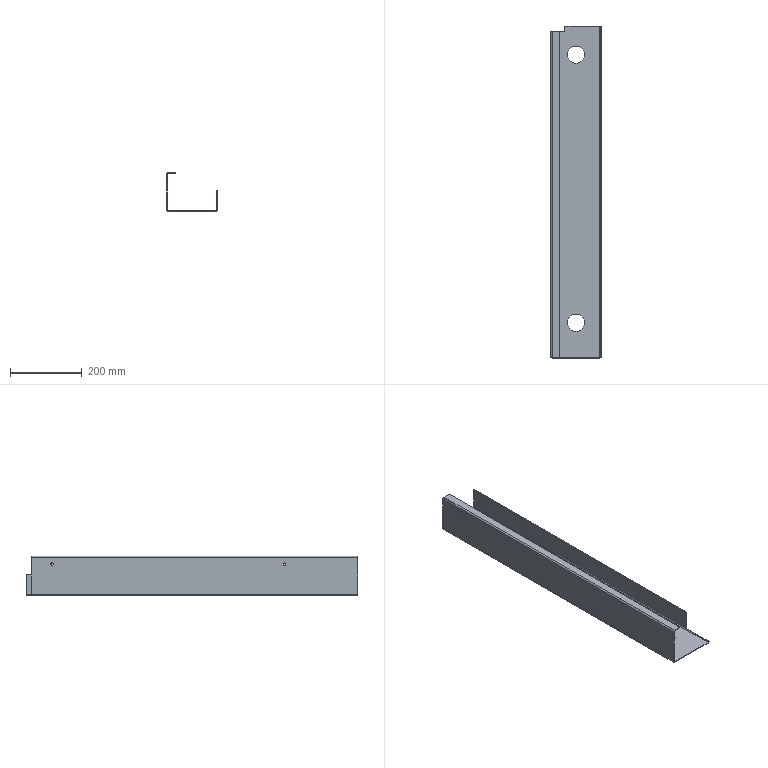Part | NX | features solid 2 | 1 solid | 30 faces | box 140 x 928 x 110 mm | volume 580849 mm3 | plane 16 | cylinder 14 | commonest cylinder face diameters 7 x4 48 x4 4 x3 8 x3
STEP:
#1=CARTESIAN_POINT('',(-1106.,-723.,1191.5));
#2=VERTEX_POINT('',#1);
#3=CARTESIAN_POINT('',(-1108.,-723.,1191.5));
#4=VERTEX_POINT('',#3);
#5=CARTESIAN_POINT('',(-2050.925,-723.,1191.5));
#6=DIRECTION('',(1.,0.,0.));
#7=VECTOR('',#6,1000.);
#8=LINE('',#5,#7);
#9=EDGE_CURVE('',#2,#4,#8,.F.);
#10=ORIENTED_EDGE('',*,*,#9,.T.);
#11=CARTESIAN_POINT('',(-1108.,-723.,1184.5));
#12=VERTEX_POINT('',#11);
#13=CARTESIAN_POINT('',(-1108.,-723.,1188.));
#14=DIRECTION('',(1.,0.,0.));
#15=DIRECTION('',(0.,0.,-1.));
#16=AXIS2_PLACEMENT_3D('',#13,#14,#15);
#17=CIRCLE('',#16,3.5);
#18=EDGE_CURVE('',#12,#4,#17,.T.);
#19=ORIENTED_EDGE('',*,*,#18,.F.);
#20=CARTESIAN_POINT('',(-1106.,-723.,1184.5));
#21=VERTEX_POINT('',#20);
#22=CARTESIAN_POINT('',(-2050.925,-723.,1184.5));
#23=DIRECTION('',(1.,0.,0.));
#24=VECTOR('',#23,1000.);
#25=LINE('',#22,#24);
#26=EDGE_CURVE('',#12,#21,#25,.T.);
#27=ORIENTED_EDGE('',*,*,#26,.T.);
#28=CARTESIAN_POINT('',(-1106.,-723.,1188.));
#29=DIRECTION('',(1.,0.,0.));
#30=DIRECTION('',(0.,1.,0.));
#31=AXIS2_PLACEMENT_3D('',#28,#29,#30);
#32=CIRCLE('',#31,3.5);
#33=EDGE_CURVE('',#21,#2,#32,.T.);
#34=ORIENTED_EDGE('',*,*,#33,.T.);
#35=EDGE_LOOP('',(#10,#19,#27,#34));
#36=FACE_BOUND('',#35,.T.);
#37=CARTESIAN_POINT('',(-2050.925,-723.,1188.));
#38=DIRECTION('',(1.,0.,0.));
#39=DIRECTION('',(0.,0.,-1.));
#40=AXIS2_PLACEMENT_3D('',#37,#38,#39);
#41=CYLINDRICAL_SURFACE('',#40,3.5);
#42=ADVANCED_FACE('',(#36),#41,.F.);
#43=CARTESIAN_POINT('',(-1106.,-1373.,1191.5));
#44=VERTEX_POINT('',#43);
#45=CARTESIAN_POINT('',(-1108.,-1373.,1191.5));
#46=VERTEX_POINT('',#45);
#47=CARTESIAN_POINT('',(-2050.925,-1373.,1191.5));
#48=DIRECTION('',(1.,0.,0.));
#49=VECTOR('',#48,1000.);
#50=LINE('',#47,#49);
#51=EDGE_CURVE('',#44,#46,#50,.F.);
#52=ORIENTED_EDGE('',*,*,#51,.T.);
#53=CARTESIAN_POINT('',(-1108.,-1373.,1184.5));
#54=VERTEX_POINT('',#53);
#55=CARTESIAN_POINT('',(-1108.,-1373.,1188.));
#56=DIRECTION('',(1.,0.,0.));
#57=DIRECTION('',(0.,0.,-1.));
#58=AXIS2_PLACEMENT_3D('',#55,#56,#57);
#59=CIRCLE('',#58,3.5);
#60=EDGE_CURVE('',#54,#46,#59,.T.);
#61=ORIENTED_EDGE('',*,*,#60,.F.);
#62=CARTESIAN_POINT('',(-1106.,-1373.,1184.5));
#63=VERTEX_POINT('',#62);
#64=CARTESIAN_POINT('',(-2050.925,-1373.,1184.5));
#65=DIRECTION('',(1.,0.,0.));
#66=VECTOR('',#65,1000.);
#67=LINE('',#64,#66);
#68=EDGE_CURVE('',#54,#63,#67,.T.);
#69=ORIENTED_EDGE('',*,*,#68,.T.);
#70=CARTESIAN_POINT('',(-1106.,-1373.,1188.));
#71=DIRECTION('',(1.,0.,0.));
#72=DIRECTION('',(0.,1.,0.));
#73=AXIS2_PLACEMENT_3D('',#70,#71,#72);
#74=CIRCLE('',#73,3.5);
#75=EDGE_CURVE('',#63,#44,#74,.T.);
#76=ORIENTED_EDGE('',*,*,#75,.T.);
#77=EDGE_LOOP('',(#52,#61,#69,#76));
#78=FACE_BOUND('',#77,.T.);
#79=CARTESIAN_POINT('',(-2050.925,-1373.,1188.));
#80=DIRECTION('',(1.,0.,0.));
#81=DIRECTION('',(0.,0.,-1.));
#82=AXIS2_PLACEMENT_3D('',#79,#80,#81);
#83=CYLINDRICAL_SURFACE('',#82,3.5);
#84=ADVANCED_FACE('',(#78),#83,.F.);
#85=CARTESIAN_POINT('',(-1106.,-666.,1206.));
#86=VERTEX_POINT('',#85);
#87=CARTESIAN_POINT('',(-1106.,-666.,1104.));
#88=VERTEX_POINT('',#87);
#89=CARTESIAN_POINT('',(-1106.,-666.,1100.));
#90=DIRECTION('',(0.,0.,-1.));
#91=VECTOR('',#90,1000.);
#92=LINE('',#89,#91);
#93=EDGE_CURVE('',#86,#88,#92,.T.);
#94=ORIENTED_EDGE('',*,*,#93,.T.);
#95=CARTESIAN_POINT('',(-1104.,-666.,1102.));
#96=VERTEX_POINT('',#95);
#97=CARTESIAN_POINT('',(-1104.,-666.,1104.));
#98=DIRECTION('',(0.,-1.,0.));
#99=DIRECTION('',(0.,0.,-1.));
#100=AXIS2_PLACEMENT_3D('',#97,#98,#99);
#101=CIRCLE('',#100,2.);
#102=EDGE_CURVE('',#88,#96,#101,.T.);
#103=ORIENTED_EDGE('',*,*,#102,.T.);
#104=CARTESIAN_POINT('',(-1069.,-666.,1102.));
#105=VERTEX_POINT('',#104);
#106=CARTESIAN_POINT('',(-968.,-666.,1102.));
#107=DIRECTION('',(1.,0.,0.));
#108=VECTOR('',#107,1000.);
#109=LINE('',#106,#108);
#110=EDGE_CURVE('',#96,#105,#109,.T.);
#111=ORIENTED_EDGE('',*,*,#110,.T.);
#112=CARTESIAN_POINT('',(-1069.,-666.,1100.));
#113=VERTEX_POINT('',#112);
#114=CARTESIAN_POINT('',(-1069.,-666.,1100.));
#115=DIRECTION('',(0.,0.,-1.));
#116=VECTOR('',#115,1000.);
#117=LINE('',#114,#116);
#118=EDGE_CURVE('',#105,#113,#117,.T.);
#119=ORIENTED_EDGE('',*,*,#118,.T.);
#120=CARTESIAN_POINT('',(-1104.,-666.,1100.));
#121=VERTEX_POINT('',#120);
#122=CARTESIAN_POINT('',(-968.,-666.,1100.));
#123=DIRECTION('',(1.,0.,0.));
#124=VECTOR('',#123,1000.);
#125=LINE('',#122,#124);
#126=EDGE_CURVE('',#121,#113,#125,.T.);
#127=ORIENTED_EDGE('',*,*,#126,.F.);
#128=CARTESIAN_POINT('',(-1108.,-666.,1104.));
#129=VERTEX_POINT('',#128);
#130=CARTESIAN_POINT('',(-1104.,-666.,1104.));
#131=DIRECTION('',(0.,-1.,0.));
#132=DIRECTION('',(0.,0.,-1.));
#133=AXIS2_PLACEMENT_3D('',#130,#131,#132);
#134=CIRCLE('',#133,4.);
#135=EDGE_CURVE('',#129,#121,#134,.T.);
#136=ORIENTED_EDGE('',*,*,#135,.F.);
#137=CARTESIAN_POINT('',(-1108.,-666.,1206.));
#138=VERTEX_POINT('',#137);
#139=CARTESIAN_POINT('',(-1108.,-666.,1100.));
#140=DIRECTION('',(0.,0.,-1.));
#141=VECTOR('',#140,1000.);
#142=LINE('',#139,#141);
#143=EDGE_CURVE('',#138,#129,#142,.T.);
#144=ORIENTED_EDGE('',*,*,#143,.F.);
#145=CARTESIAN_POINT('',(-1104.,-666.,1210.));
#146=VERTEX_POINT('',#145);
#147=CARTESIAN_POINT('',(-1104.,-666.,1206.));
#148=DIRECTION('',(0.,-1.,0.));
#149=DIRECTION('',(0.,0.,-1.));
#150=AXIS2_PLACEMENT_3D('',#147,#148,#149);
#151=CIRCLE('',#150,4.);
#152=EDGE_CURVE('',#146,#138,#151,.T.);
#153=ORIENTED_EDGE('',*,*,#152,.F.);
#154=CARTESIAN_POINT('',(-1083.,-666.,1210.));
#155=VERTEX_POINT('',#154);
#156=CARTESIAN_POINT('',(-1108.,-666.,1210.));
#157=DIRECTION('',(-1.,0.,0.));
#158=VECTOR('',#157,1000.);
#159=LINE('',#156,#158);
#160=EDGE_CURVE('',#155,#146,#159,.T.);
#161=ORIENTED_EDGE('',*,*,#160,.F.);
#162=CARTESIAN_POINT('',(-1083.,-666.,1208.));
#163=VERTEX_POINT('',#162);
#164=CARTESIAN_POINT('',(-1083.,-666.,1210.));
#165=DIRECTION('',(0.,0.,1.));
#166=VECTOR('',#165,1000.);
#167=LINE('',#164,#166);
#168=EDGE_CURVE('',#163,#155,#167,.T.);
#169=ORIENTED_EDGE('',*,*,#168,.F.);
#170=CARTESIAN_POINT('',(-1104.,-666.,1208.));
#171=VERTEX_POINT('',#170);
#172=CARTESIAN_POINT('',(-1108.,-666.,1208.));
#173=DIRECTION('',(-1.,0.,0.));
#174=VECTOR('',#173,1000.);
#175=LINE('',#172,#174);
#176=EDGE_CURVE('',#163,#171,#175,.T.);
#177=ORIENTED_EDGE('',*,*,#176,.T.);
#178=CARTESIAN_POINT('',(-1104.,-666.,1206.));
#179=DIRECTION('',(0.,-1.,0.));
#180=DIRECTION('',(0.,0.,-1.));
#181=AXIS2_PLACEMENT_3D('',#178,#179,#180);
#182=CIRCLE('',#181,2.);
#183=EDGE_CURVE('',#171,#86,#182,.T.);
#184=ORIENTED_EDGE('',*,*,#183,.T.);
#185=EDGE_LOOP('',(#94,#103,#111,#119,#127,#136,#144,#153,#161,#169,#177,#184));
#186=FACE_BOUND('',#185,.T.);
#187=CARTESIAN_POINT('',(-1108.,-666.,1100.));
#188=DIRECTION('',(0.,-1.,0.));
#189=DIRECTION('',(0.,0.,-1.));
#190=AXIS2_PLACEMENT_3D('',#187,#188,#189);
#191=PLANE('',#190);
#192=ADVANCED_FACE('',(#186),#191,.F.);
#193=CARTESIAN_POINT('',(-1069.,-650.,1102.));
#194=VERTEX_POINT('',#193);
#195=CARTESIAN_POINT('',(-1069.,-650.,1100.));
#196=VERTEX_POINT('',#195);
#197=CARTESIAN_POINT('',(-1069.,-650.,1100.));
#198=DIRECTION('',(0.,0.,-1.));
#199=VECTOR('',#198,1000.);
#200=LINE('',#197,#199);
#201=EDGE_CURVE('',#194,#196,#200,.T.);
#202=ORIENTED_EDGE('',*,*,#201,.T.);
#203=CARTESIAN_POINT('',(-1069.,-650.,1100.));
#204=DIRECTION('',(0.,1.,0.));
#205=VECTOR('',#204,1000.);
#206=LINE('',#203,#205);
#207=EDGE_CURVE('',#113,#196,#206,.T.);
#208=ORIENTED_EDGE('',*,*,#207,.F.);
#209=ORIENTED_EDGE('',*,*,#118,.F.);
#210=CARTESIAN_POINT('',(-1069.,-650.,1102.));
#211=DIRECTION('',(0.,1.,0.));
#212=VECTOR('',#211,1000.);
#213=LINE('',#210,#212);
#214=EDGE_CURVE('',#105,#194,#213,.T.);
#215=ORIENTED_EDGE('',*,*,#214,.T.);
#216=EDGE_LOOP('',(#202,#208,#209,#215));
#217=FACE_BOUND('',#216,.T.);
#218=CARTESIAN_POINT('',(-1069.,-650.,1100.));
#219=DIRECTION('',(1.,0.,0.));
#220=DIRECTION('',(0.,1.,0.));
#221=AXIS2_PLACEMENT_3D('',#218,#219,#220);
#222=PLANE('',#221);
#223=ADVANCED_FACE('',(#217),#222,.F.);
#224=CARTESIAN_POINT('',(-970.,-1490.,1160.));
#225=VERTEX_POINT('',#224);
#226=CARTESIAN_POINT('',(-970.,-1490.,1104.));
#227=VERTEX_POINT('',#226);
#228=CARTESIAN_POINT('',(-970.,-1490.,1160.));
#229=DIRECTION('',(0.,0.,-1.));
#230=VECTOR('',#229,1000.);
#231=LINE('',#228,#230);
#232=EDGE_CURVE('',#225,#227,#231,.T.);
#233=ORIENTED_EDGE('',*,*,#232,.T.);
#234=CARTESIAN_POINT('',(-968.,-1490.,1104.));
#235=VERTEX_POINT('',#234);
#236=CARTESIAN_POINT('',(-968.,-1490.,1104.));
#237=DIRECTION('',(1.,0.,0.));
#238=VECTOR('',#237,1000.);
#239=LINE('',#236,#238);
#240=EDGE_CURVE('',#227,#235,#239,.T.);
#241=ORIENTED_EDGE('',*,*,#240,.T.);
#242=CARTESIAN_POINT('',(-968.,-1490.,1160.));
#243=VERTEX_POINT('',#242);
#244=CARTESIAN_POINT('',(-968.,-1490.,1160.));
#245=DIRECTION('',(0.,0.,-1.));
#246=VECTOR('',#245,1000.);
#247=LINE('',#244,#246);
#248=EDGE_CURVE('',#243,#235,#247,.T.);
#249=ORIENTED_EDGE('',*,*,#248,.F.);
#250=CARTESIAN_POINT('',(-968.,-1490.,1160.));
#251=DIRECTION('',(1.,0.,0.));
#252=VECTOR('',#251,1000.);
#253=LINE('',#250,#252);
#254=EDGE_CURVE('',#225,#243,#253,.T.);
#255=ORIENTED_EDGE('',*,*,#254,.F.);
#256=EDGE_LOOP('',(#233,#241,#249,#255));
#257=FACE_BOUND('',#256,.T.);
#258=CARTESIAN_POINT('',(-968.,-1490.,1160.));
#259=DIRECTION('',(0.,1.,0.));
#260=DIRECTION('',(1.,0.,0.));
#261=AXIS2_PLACEMENT_3D('',#258,#259,#260);
#262=PLANE('',#261);
#263=ADVANCED_FACE('',(#257),#262,.F.);
#264=CARTESIAN_POINT('',(-970.,-1578.,1104.));
#265=VERTEX_POINT('',#264);
#266=CARTESIAN_POINT('',(-968.,-1578.,1104.));
#267=VERTEX_POINT('',#266);
#268=CARTESIAN_POINT('',(-968.,-1578.,1104.));
#269=DIRECTION('',(1.,0.,0.));
#270=VECTOR('',#269,1000.);
#271=LINE('',#268,#270);
#272=EDGE_CURVE('',#265,#267,#271,.T.);
#273=ORIENTED_EDGE('',*,*,#272,.T.);
#274=CARTESIAN_POINT('',(-968.,-650.,1104.));
#275=DIRECTION('',(0.,-1.,0.));
#276=VECTOR('',#275,1000.);
#277=LINE('',#274,#276);
#278=EDGE_CURVE('',#235,#267,#277,.T.);
#279=ORIENTED_EDGE('',*,*,#278,.F.);
#280=ORIENTED_EDGE('',*,*,#240,.F.);
#281=CARTESIAN_POINT('',(-970.,-650.,1104.));
#282=DIRECTION('',(0.,-1.,0.));
#283=VECTOR('',#282,1000.);
#284=LINE('',#281,#283);
#285=EDGE_CURVE('',#227,#265,#284,.T.);
#286=ORIENTED_EDGE('',*,*,#285,.T.);
#287=EDGE_LOOP('',(#273,#279,#280,#286));
#288=FACE_BOUND('',#287,.T.);
#289=CARTESIAN_POINT('',(-968.,-650.,1104.));
#290=DIRECTION('',(0.,0.,-1.));
#291=DIRECTION('',(0.,-1.,0.));
#292=AXIS2_PLACEMENT_3D('',#289,#290,#291);
#293=PLANE('',#292);
#294=ADVANCED_FACE('',(#288),#293,.F.);
#295=CARTESIAN_POINT('',(-1014.,-730.,1102.));
#296=VERTEX_POINT('',#295);
#297=CARTESIAN_POINT('',(-1014.,-730.,1100.));
#298=VERTEX_POINT('',#297);
#299=CARTESIAN_POINT('',(-1014.,-730.,2044.925));
#300=DIRECTION('',(0.,0.,-1.));
#301=VECTOR('',#300,1000.);
#302=LINE('',#299,#301);
#303=EDGE_CURVE('',#296,#298,#302,.T.);
#304=ORIENTED_EDGE('',*,*,#303,.F.);
#305=CARTESIAN_POINT('',(-1062.,-730.,1102.));
#306=VERTEX_POINT('',#305);
#307=CARTESIAN_POINT('',(-1038.,-730.,1102.));
#308=DIRECTION('',(0.,0.,1.));
#309=DIRECTION('',(1.,0.,0.));
#310=AXIS2_PLACEMENT_3D('',#307,#308,#309);
#311=CIRCLE('',#310,24.);
#312=EDGE_CURVE('',#296,#306,#311,.T.);
#313=ORIENTED_EDGE('',*,*,#312,.T.);
#314=CARTESIAN_POINT('',(-1062.,-730.,1100.));
#315=VERTEX_POINT('',#314);
#316=CARTESIAN_POINT('',(-1062.,-730.,2044.925));
#317=DIRECTION('',(0.,0.,-1.));
#318=VECTOR('',#317,1000.);
#319=LINE('',#316,#318);
#320=EDGE_CURVE('',#315,#306,#319,.F.);
#321=ORIENTED_EDGE('',*,*,#320,.F.);
#322=CARTESIAN_POINT('',(-1038.,-730.,1100.));
#323=DIRECTION('',(0.,0.,-1.));
#324=DIRECTION('',(0.,-1.,0.));
#325=AXIS2_PLACEMENT_3D('',#322,#323,#324);
#326=CIRCLE('',#325,24.);
#327=EDGE_CURVE('',#315,#298,#326,.T.);
#328=ORIENTED_EDGE('',*,*,#327,.T.);
#329=EDGE_LOOP('',(#304,#313,#321,#328));
#330=FACE_BOUND('',#329,.T.);
#331=CARTESIAN_POINT('',(-1038.,-730.,2044.925));
#332=DIRECTION('',(0.,0.,-1.));
#333=DIRECTION('',(-1.,0.,0.));
#334=AXIS2_PLACEMENT_3D('',#331,#332,#333);
#335=CYLINDRICAL_SURFACE('',#334,24.);
#336=ADVANCED_FACE('',(#330),#335,.F.);
#337=CARTESIAN_POINT('',(-1014.,-1480.,1102.));
#338=VERTEX_POINT('',#337);
#339=CARTESIAN_POINT('',(-1014.,-1480.,1100.));
#340=VERTEX_POINT('',#339);
#341=CARTESIAN_POINT('',(-1014.,-1480.,2044.925));
#342=DIRECTION('',(0.,0.,-1.));
#343=VECTOR('',#342,1000.);
#344=LINE('',#341,#343);
#345=EDGE_CURVE('',#338,#340,#344,.T.);
#346=ORIENTED_EDGE('',*,*,#345,.F.);
#347=CARTESIAN_POINT('',(-1062.,-1480.,1102.));
#348=VERTEX_POINT('',#347);
#349=CARTESIAN_POINT('',(-1038.,-1480.,1102.));
#350=DIRECTION('',(0.,0.,1.));
#351=DIRECTION('',(1.,0.,0.));
#352=AXIS2_PLACEMENT_3D('',#349,#350,#351);
#353=CIRCLE('',#352,24.);
#354=EDGE_CURVE('',#338,#348,#353,.T.);
#355=ORIENTED_EDGE('',*,*,#354,.T.);
#356=CARTESIAN_POINT('',(-1062.,-1480.,1100.));
#357=VERTEX_POINT('',#356);
#358=CARTESIAN_POINT('',(-1062.,-1480.,2044.925));
#359=DIRECTION('',(0.,0.,-1.));
#360=VECTOR('',#359,1000.);
#361=LINE('',#358,#360);
#362=EDGE_CURVE('',#357,#348,#361,.F.);
#363=ORIENTED_EDGE('',*,*,#362,.F.);
#364=CARTESIAN_POINT('',(-1038.,-1480.,1100.));
#365=DIRECTION('',(0.,0.,-1.));
#366=DIRECTION('',(0.,-1.,0.));
#367=AXIS2_PLACEMENT_3D('',#364,#365,#366);
#368=CIRCLE('',#367,24.);
#369=EDGE_CURVE('',#357,#340,#368,.T.);
#370=ORIENTED_EDGE('',*,*,#369,.T.);
#371=EDGE_LOOP('',(#346,#355,#363,#370));
#372=FACE_BOUND('',#371,.T.);
#373=CARTESIAN_POINT('',(-1038.,-1480.,2044.925));
#374=DIRECTION('',(0.,0.,-1.));
#375=DIRECTION('',(-1.,0.,0.));
#376=AXIS2_PLACEMENT_3D('',#373,#374,#375);
#377=CYLINDRICAL_SURFACE('',#376,24.);
#378=ADVANCED_FACE('',(#372),#377,.F.);
#379=CARTESIAN_POINT('',(-1083.,-1578.,1210.));
#380=VERTEX_POINT('',#379);
#381=CARTESIAN_POINT('',(-1083.,-650.,1210.));
#382=DIRECTION('',(0.,-1.,0.));
#383=VECTOR('',#382,1000.);
#384=LINE('',#381,#383);
#385=EDGE_CURVE('',#155,#380,#384,.T.);
#386=ORIENTED_EDGE('',*,*,#385,.F.);
#387=ORIENTED_EDGE('',*,*,#160,.T.);
#388=CARTESIAN_POINT('',(-1104.,-1578.,1210.));
#389=VERTEX_POINT('',#388);
#390=CARTESIAN_POINT('',(-1104.,-650.,1210.));
#391=DIRECTION('',(0.,-1.,0.));
#392=VECTOR('',#391,1000.);
#393=LINE('',#390,#392);
#394=EDGE_CURVE('',#146,#389,#393,.T.);
#395=ORIENTED_EDGE('',*,*,#394,.T.);
#396=CARTESIAN_POINT('',(-1108.,-1578.,1210.));
#397=DIRECTION('',(1.,0.,0.));
#398=VECTOR('',#397,1000.);
#399=LINE('',#396,#398);
#400=EDGE_CURVE('',#389,#380,#399,.T.);
#401=ORIENTED_EDGE('',*,*,#400,.T.);
#402=EDGE_LOOP('',(#386,#387,#395,#401));
#403=FACE_BOUND('',#402,.T.);
#404=CARTESIAN_POINT('',(-1108.,-650.,1210.));
#405=DIRECTION('',(0.,0.,-1.));
#406=DIRECTION('',(0.,-1.,0.));
#407=AXIS2_PLACEMENT_3D('',#404,#405,#406);
#408=PLANE('',#407);
#409=ADVANCED_FACE('',(#403),#408,.F.);
#410=ORIENTED_EDGE('',*,*,#394,.F.);
#411=ORIENTED_EDGE('',*,*,#152,.T.);
#412=CARTESIAN_POINT('',(-1108.,-1578.,1206.));
#413=VERTEX_POINT('',#412);
#414=CARTESIAN_POINT('',(-1108.,-650.,1206.));
#415=DIRECTION('',(0.,-1.,0.));
#416=VECTOR('',#415,1000.);
#417=LINE('',#414,#416);
#418=EDGE_CURVE('',#138,#413,#417,.T.);
#419=ORIENTED_EDGE('',*,*,#418,.T.);
#420=CARTESIAN_POINT('',(-1104.,-1578.,1206.));
#421=DIRECTION('',(0.,1.,0.));
#422=DIRECTION('',(0.,0.,-1.));
#423=AXIS2_PLACEMENT_3D('',#420,#421,#422);
#424=CIRCLE('',#423,4.);
#425=EDGE_CURVE('',#413,#389,#424,.T.);
#426=ORIENTED_EDGE('',*,*,#425,.T.);
#427=EDGE_LOOP('',(#410,#411,#419,#426));
#428=FACE_BOUND('',#427,.T.);
#429=CARTESIAN_POINT('',(-1104.,-650.,1206.));
#430=DIRECTION('',(0.,-1.,0.));
#431=DIRECTION('',(0.,0.,-1.));
#432=AXIS2_PLACEMENT_3D('',#429,#430,#431);
#433=CYLINDRICAL_SURFACE('',#432,4.);
#434=ADVANCED_FACE('',(#428),#433,.T.);
#435=ORIENTED_EDGE('',*,*,#60,.T.);
#436=CARTESIAN_POINT('',(-1108.,-1373.,1188.));
#437=DIRECTION('',(1.,0.,0.));
#438=DIRECTION('',(0.,0.,-1.));
#439=AXIS2_PLACEMENT_3D('',#436,#437,#438);
#440=CIRCLE('',#439,3.5);
#441=EDGE_CURVE('',#46,#54,#440,.T.);
#442=ORIENTED_EDGE('',*,*,#441,.T.);
#443=EDGE_LOOP('',(#435,#442));
#444=FACE_BOUND('',#443,.T.);
#445=ORIENTED_EDGE('',*,*,#18,.T.);
#446=CARTESIAN_POINT('',(-1108.,-723.,1188.));
#447=DIRECTION('',(1.,0.,0.));
#448=DIRECTION('',(0.,0.,-1.));
#449=AXIS2_PLACEMENT_3D('',#446,#447,#448);
#450=CIRCLE('',#449,3.5);
#451=EDGE_CURVE('',#4,#12,#450,.T.);
#452=ORIENTED_EDGE('',*,*,#451,.T.);
#453=EDGE_LOOP('',(#445,#452));
#454=FACE_BOUND('',#453,.T.);
#455=ORIENTED_EDGE('',*,*,#418,.F.);
#456=ORIENTED_EDGE('',*,*,#143,.T.);
#457=CARTESIAN_POINT('',(-1108.,-1578.,1104.));
#458=VERTEX_POINT('',#457);
#459=CARTESIAN_POINT('',(-1108.,-650.,1104.));
#460=DIRECTION('',(0.,-1.,0.));
#461=VECTOR('',#460,1000.);
#462=LINE('',#459,#461);
#463=EDGE_CURVE('',#129,#458,#462,.T.);
#464=ORIENTED_EDGE('',*,*,#463,.T.);
#465=CARTESIAN_POINT('',(-1108.,-1578.,1100.));
#466=DIRECTION('',(0.,0.,1.));
#467=VECTOR('',#466,1000.);
#468=LINE('',#465,#467);
#469=EDGE_CURVE('',#458,#413,#468,.T.);
#470=ORIENTED_EDGE('',*,*,#469,.T.);
#471=EDGE_LOOP('',(#455,#456,#464,#470));
#472=FACE_BOUND('',#471,.T.);
#473=CARTESIAN_POINT('',(-1108.,-650.,1100.));
#474=DIRECTION('',(1.,0.,0.));
#475=DIRECTION('',(0.,1.,0.));
#476=AXIS2_PLACEMENT_3D('',#473,#474,#475);
#477=PLANE('',#476);
#478=ADVANCED_FACE('',(#444,#454,#472),#477,.F.);
#479=ORIENTED_EDGE('',*,*,#463,.F.);
#480=ORIENTED_EDGE('',*,*,#135,.T.);
#481=CARTESIAN_POINT('',(-1104.,-1578.,1100.));
#482=VERTEX_POINT('',#481);
#483=CARTESIAN_POINT('',(-1104.,-650.,1100.));
#484=DIRECTION('',(0.,-1.,0.));
#485=VECTOR('',#484,1000.);
#486=LINE('',#483,#485);
#487=EDGE_CURVE('',#121,#482,#486,.T.);
#488=ORIENTED_EDGE('',*,*,#487,.T.);
#489=CARTESIAN_POINT('',(-1104.,-1578.,1104.));
#490=DIRECTION('',(0.,1.,0.));
#491=DIRECTION('',(0.,0.,-1.));
#492=AXIS2_PLACEMENT_3D('',#489,#490,#491);
#493=CIRCLE('',#492,4.);
#494=EDGE_CURVE('',#482,#458,#493,.T.);
#495=ORIENTED_EDGE('',*,*,#494,.T.);
#496=EDGE_LOOP('',(#479,#480,#488,#495));
#497=FACE_BOUND('',#496,.T.);
#498=CARTESIAN_POINT('',(-1104.,-650.,1104.));
#499=DIRECTION('',(0.,-1.,0.));
#500=DIRECTION('',(0.,0.,-1.));
#501=AXIS2_PLACEMENT_3D('',#498,#499,#500);
#502=CYLINDRICAL_SURFACE('',#501,4.);
#503=ADVANCED_FACE('',(#497),#502,.T.);
#504=ORIENTED_EDGE('',*,*,#369,.F.);
#505=CARTESIAN_POINT('',(-1038.,-1480.,1100.));
#506=DIRECTION('',(0.,0.,-1.));
#507=DIRECTION('',(0.,-1.,0.));
#508=AXIS2_PLACEMENT_3D('',#505,#506,#507);
#509=CIRCLE('',#508,24.);
#510=EDGE_CURVE('',#340,#357,#509,.T.);
#511=ORIENTED_EDGE('',*,*,#510,.F.);
#512=EDGE_LOOP('',(#504,#511));
#513=FACE_BOUND('',#512,.T.);
#514=ORIENTED_EDGE('',*,*,#327,.F.);
#515=CARTESIAN_POINT('',(-1038.,-730.,1100.));
#516=DIRECTION('',(0.,0.,-1.));
#517=DIRECTION('',(0.,-1.,0.));
#518=AXIS2_PLACEMENT_3D('',#515,#516,#517);
#519=CIRCLE('',#518,24.);
#520=EDGE_CURVE('',#298,#315,#519,.T.);
#521=ORIENTED_EDGE('',*,*,#520,.F.);
#522=EDGE_LOOP('',(#514,#521));
#523=FACE_BOUND('',#522,.T.);
#524=ORIENTED_EDGE('',*,*,#126,.T.);
#525=ORIENTED_EDGE('',*,*,#207,.T.);
#526=CARTESIAN_POINT('',(-972.,-650.,1100.));
#527=VERTEX_POINT('',#526);
#528=CARTESIAN_POINT('',(-968.,-650.,1100.));
#529=DIRECTION('',(-1.,0.,0.));
#530=VECTOR('',#529,1000.);
#531=LINE('',#528,#530);
#532=EDGE_CURVE('',#527,#196,#531,.T.);
#533=ORIENTED_EDGE('',*,*,#532,.F.);
#534=CARTESIAN_POINT('',(-972.,-1578.,1100.));
#535=VERTEX_POINT('',#534);
#536=CARTESIAN_POINT('',(-972.,-650.,1100.));
#537=DIRECTION('',(0.,-1.,0.));
#538=VECTOR('',#537,1000.);
#539=LINE('',#536,#538);
#540=EDGE_CURVE('',#527,#535,#539,.T.);
#541=ORIENTED_EDGE('',*,*,#540,.T.);
#542=CARTESIAN_POINT('',(-968.,-1578.,1100.));
#543=DIRECTION('',(-1.,0.,0.));
#544=VECTOR('',#543,1000.);
#545=LINE('',#542,#544);
#546=EDGE_CURVE('',#535,#482,#545,.T.);
#547=ORIENTED_EDGE('',*,*,#546,.T.);
#548=ORIENTED_EDGE('',*,*,#487,.F.);
#549=EDGE_LOOP('',(#524,#525,#533,#541,#547,#548));
#550=FACE_BOUND('',#549,.T.);
#551=CARTESIAN_POINT('',(-968.,-650.,1100.));
#552=DIRECTION('',(0.,0.,1.));
#553=DIRECTION('',(1.,0.,0.));
#554=AXIS2_PLACEMENT_3D('',#551,#552,#553);
#555=PLANE('',#554);
#556=ADVANCED_FACE('',(#513,#523,#550),#555,.F.);
#557=CARTESIAN_POINT('',(-972.,-1578.,1104.));
#558=DIRECTION('',(0.,1.,0.));
#559=DIRECTION('',(0.,0.,-1.));
#560=AXIS2_PLACEMENT_3D('',#557,#558,#559);
#561=CIRCLE('',#560,4.);
#562=EDGE_CURVE('',#267,#535,#561,.T.);
#563=ORIENTED_EDGE('',*,*,#562,.T.);
#564=ORIENTED_EDGE('',*,*,#540,.F.);
#565=CARTESIAN_POINT('',(-968.,-650.,1104.));
#566=VERTEX_POINT('',#565);
#567=CARTESIAN_POINT('',(-972.,-650.,1104.));
#568=DIRECTION('',(0.,1.,0.));
#569=DIRECTION('',(0.,0.,-1.));
#570=AXIS2_PLACEMENT_3D('',#567,#568,#569);
#571=CIRCLE('',#570,4.);
#572=EDGE_CURVE('',#566,#527,#571,.T.);
#573=ORIENTED_EDGE('',*,*,#572,.F.);
#574=CARTESIAN_POINT('',(-968.,-650.,1104.));
#575=DIRECTION('',(0.,-1.,0.));
#576=VECTOR('',#575,1000.);
#577=LINE('',#574,#576);
#578=EDGE_CURVE('',#566,#235,#577,.T.);
#579=ORIENTED_EDGE('',*,*,#578,.T.);
#580=ORIENTED_EDGE('',*,*,#278,.T.);
#581=EDGE_LOOP('',(#563,#564,#573,#579,#580));
#582=FACE_BOUND('',#581,.T.);
#583=CARTESIAN_POINT('',(-972.,-650.,1104.));
#584=DIRECTION('',(0.,-1.,0.));
#585=DIRECTION('',(0.,0.,-1.));
#586=AXIS2_PLACEMENT_3D('',#583,#584,#585);
#587=CYLINDRICAL_SURFACE('',#586,4.);
#588=ADVANCED_FACE('',(#582),#587,.T.);
#589=CARTESIAN_POINT('',(-968.,-650.,1160.));
#590=VERTEX_POINT('',#589);
#591=CARTESIAN_POINT('',(-968.,-650.,1160.));
#592=DIRECTION('',(0.,-1.,0.));
#593=VECTOR('',#592,1000.);
#594=LINE('',#591,#593);
#595=EDGE_CURVE('',#590,#243,#594,.T.);
#596=ORIENTED_EDGE('',*,*,#595,.T.);
#597=ORIENTED_EDGE('',*,*,#248,.T.);
#598=ORIENTED_EDGE('',*,*,#578,.F.);
#599=CARTESIAN_POINT('',(-968.,-650.,1160.));
#600=DIRECTION('',(0.,0.,-1.));
#601=VECTOR('',#600,1000.);
#602=LINE('',#599,#601);
#603=EDGE_CURVE('',#590,#566,#602,.T.);
#604=ORIENTED_EDGE('',*,*,#603,.F.);
#605=EDGE_LOOP('',(#596,#597,#598,#604));
#606=FACE_BOUND('',#605,.T.);
#607=CARTESIAN_POINT('',(-968.,-650.,1160.));
#608=DIRECTION('',(-1.,0.,0.));
#609=DIRECTION('',(0.,0.,1.));
#610=AXIS2_PLACEMENT_3D('',#607,#608,#609);
#611=PLANE('',#610);
#612=ADVANCED_FACE('',(#606),#611,.F.);
#613=ORIENTED_EDGE('',*,*,#176,.F.);
#614=CARTESIAN_POINT('',(-1083.,-1578.,1208.));
#615=VERTEX_POINT('',#614);
#616=CARTESIAN_POINT('',(-1083.,-650.,1208.));
#617=DIRECTION('',(0.,-1.,0.));
#618=VECTOR('',#617,1000.);
#619=LINE('',#616,#618);
#620=EDGE_CURVE('',#163,#615,#619,.T.);
#621=ORIENTED_EDGE('',*,*,#620,.T.);
#622=CARTESIAN_POINT('',(-1104.,-1578.,1208.));
#623=VERTEX_POINT('',#622);
#624=CARTESIAN_POINT('',(-1108.,-1578.,1208.));
#625=DIRECTION('',(1.,0.,0.));
#626=VECTOR('',#625,1000.);
#627=LINE('',#624,#626);
#628=EDGE_CURVE('',#623,#615,#627,.T.);
#629=ORIENTED_EDGE('',*,*,#628,.F.);
#630=CARTESIAN_POINT('',(-1104.,-650.,1208.));
#631=DIRECTION('',(0.,-1.,0.));
#632=VECTOR('',#631,1000.);
#633=LINE('',#630,#632);
#634=EDGE_CURVE('',#171,#623,#633,.T.);
#635=ORIENTED_EDGE('',*,*,#634,.F.);
#636=EDGE_LOOP('',(#613,#621,#629,#635));
#637=FACE_BOUND('',#636,.T.);
#638=CARTESIAN_POINT('',(-1108.,-650.,1208.));
#639=DIRECTION('',(0.,0.,-1.));
#640=DIRECTION('',(0.,-1.,0.));
#641=AXIS2_PLACEMENT_3D('',#638,#639,#640);
#642=PLANE('',#641);
#643=ADVANCED_FACE('',(#637),#642,.T.);
#644=ORIENTED_EDGE('',*,*,#183,.F.);
#645=ORIENTED_EDGE('',*,*,#634,.T.);
#646=CARTESIAN_POINT('',(-1106.,-1578.,1206.));
#647=VERTEX_POINT('',#646);
#648=CARTESIAN_POINT('',(-1104.,-1578.,1206.));
#649=DIRECTION('',(0.,1.,0.));
#650=DIRECTION('',(0.,0.,-1.));
#651=AXIS2_PLACEMENT_3D('',#648,#649,#650);
#652=CIRCLE('',#651,2.);
#653=EDGE_CURVE('',#647,#623,#652,.T.);
#654=ORIENTED_EDGE('',*,*,#653,.F.);
#655=CARTESIAN_POINT('',(-1106.,-650.,1206.));
#656=DIRECTION('',(0.,-1.,0.));
#657=VECTOR('',#656,1000.);
#658=LINE('',#655,#657);
#659=EDGE_CURVE('',#86,#647,#658,.T.);
#660=ORIENTED_EDGE('',*,*,#659,.F.);
#661=EDGE_LOOP('',(#644,#645,#654,#660));
#662=FACE_BOUND('',#661,.T.);
#663=CARTESIAN_POINT('',(-1104.,-650.,1206.));
#664=DIRECTION('',(0.,-1.,0.));
#665=DIRECTION('',(0.,0.,-1.));
#666=AXIS2_PLACEMENT_3D('',#663,#664,#665);
#667=CYLINDRICAL_SURFACE('',#666,2.);
#668=ADVANCED_FACE('',(#662),#667,.F.);
#669=ORIENTED_EDGE('',*,*,#75,.F.);
#670=CARTESIAN_POINT('',(-1106.,-1373.,1188.));
#671=DIRECTION('',(1.,0.,0.));
#672=DIRECTION('',(0.,1.,0.));
#673=AXIS2_PLACEMENT_3D('',#670,#671,#672);
#674=CIRCLE('',#673,3.5);
#675=EDGE_CURVE('',#44,#63,#674,.T.);
#676=ORIENTED_EDGE('',*,*,#675,.F.);
#677=EDGE_LOOP('',(#669,#676));
#678=FACE_BOUND('',#677,.T.);
#679=ORIENTED_EDGE('',*,*,#33,.F.);
#680=CARTESIAN_POINT('',(-1106.,-723.,1188.));
#681=DIRECTION('',(1.,0.,0.));
#682=DIRECTION('',(0.,1.,0.));
#683=AXIS2_PLACEMENT_3D('',#680,#681,#682);
#684=CIRCLE('',#683,3.5);
#685=EDGE_CURVE('',#2,#21,#684,.T.);
#686=ORIENTED_EDGE('',*,*,#685,.F.);
#687=EDGE_LOOP('',(#679,#686));
#688=FACE_BOUND('',#687,.T.);
#689=ORIENTED_EDGE('',*,*,#93,.F.);
#690=ORIENTED_EDGE('',*,*,#659,.T.);
#691=CARTESIAN_POINT('',(-1106.,-1578.,1104.));
#692=VERTEX_POINT('',#691);
#693=CARTESIAN_POINT('',(-1106.,-1578.,1100.));
#694=DIRECTION('',(0.,0.,1.));
#695=VECTOR('',#694,1000.);
#696=LINE('',#693,#695);
#697=EDGE_CURVE('',#692,#647,#696,.T.);
#698=ORIENTED_EDGE('',*,*,#697,.F.);
#699=CARTESIAN_POINT('',(-1106.,-650.,1104.));
#700=DIRECTION('',(0.,-1.,0.));
#701=VECTOR('',#700,1000.);
#702=LINE('',#699,#701);
#703=EDGE_CURVE('',#88,#692,#702,.T.);
#704=ORIENTED_EDGE('',*,*,#703,.F.);
#705=EDGE_LOOP('',(#689,#690,#698,#704));
#706=FACE_BOUND('',#705,.T.);
#707=CARTESIAN_POINT('',(-1106.,-650.,1100.));
#708=DIRECTION('',(1.,0.,0.));
#709=DIRECTION('',(0.,1.,0.));
#710=AXIS2_PLACEMENT_3D('',#707,#708,#709);
#711=PLANE('',#710);
#712=ADVANCED_FACE('',(#678,#688,#706),#711,.T.);
#713=ORIENTED_EDGE('',*,*,#102,.F.);
#714=ORIENTED_EDGE('',*,*,#703,.T.);
#715=CARTESIAN_POINT('',(-1104.,-1578.,1102.));
#716=VERTEX_POINT('',#715);
#717=CARTESIAN_POINT('',(-1104.,-1578.,1104.));
#718=DIRECTION('',(0.,1.,0.));
#719=DIRECTION('',(0.,0.,-1.));
#720=AXIS2_PLACEMENT_3D('',#717,#718,#719);
#721=CIRCLE('',#720,2.);
#722=EDGE_CURVE('',#716,#692,#721,.T.);
#723=ORIENTED_EDGE('',*,*,#722,.F.);
#724=CARTESIAN_POINT('',(-1104.,-650.,1102.));
#725=DIRECTION('',(0.,-1.,0.));
#726=VECTOR('',#725,1000.);
#727=LINE('',#724,#726);
#728=EDGE_CURVE('',#96,#716,#727,.T.);
#729=ORIENTED_EDGE('',*,*,#728,.F.);
#730=EDGE_LOOP('',(#713,#714,#723,#729));
#731=FACE_BOUND('',#730,.T.);
#732=CARTESIAN_POINT('',(-1104.,-650.,1104.));
#733=DIRECTION('',(0.,-1.,0.));
#734=DIRECTION('',(0.,0.,-1.));
#735=AXIS2_PLACEMENT_3D('',#732,#733,#734);
#736=CYLINDRICAL_SURFACE('',#735,2.);
#737=ADVANCED_FACE('',(#731),#736,.F.);
#738=CARTESIAN_POINT('',(-1038.,-1480.,1102.));
#739=DIRECTION('',(0.,0.,1.));
#740=DIRECTION('',(1.,0.,0.));
#741=AXIS2_PLACEMENT_3D('',#738,#739,#740);
#742=CIRCLE('',#741,24.);
#743=EDGE_CURVE('',#348,#338,#742,.T.);
#744=ORIENTED_EDGE('',*,*,#743,.F.);
#745=ORIENTED_EDGE('',*,*,#354,.F.);
#746=EDGE_LOOP('',(#744,#745));
#747=FACE_BOUND('',#746,.T.);
#748=CARTESIAN_POINT('',(-1038.,-730.,1102.));
#749=DIRECTION('',(0.,0.,1.));
#750=DIRECTION('',(1.,0.,0.));
#751=AXIS2_PLACEMENT_3D('',#748,#749,#750);
#752=CIRCLE('',#751,24.);
#753=EDGE_CURVE('',#306,#296,#752,.T.);
#754=ORIENTED_EDGE('',*,*,#753,.F.);
#755=ORIENTED_EDGE('',*,*,#312,.F.);
#756=EDGE_LOOP('',(#754,#755));
#757=FACE_BOUND('',#756,.T.);
#758=ORIENTED_EDGE('',*,*,#214,.F.);
#759=ORIENTED_EDGE('',*,*,#110,.F.);
#760=ORIENTED_EDGE('',*,*,#728,.T.);
#761=CARTESIAN_POINT('',(-972.,-1578.,1102.));
#762=VERTEX_POINT('',#761);
#763=CARTESIAN_POINT('',(-968.,-1578.,1102.));
#764=DIRECTION('',(-1.,0.,0.));
#765=VECTOR('',#764,1000.);
#766=LINE('',#763,#765);
#767=EDGE_CURVE('',#762,#716,#766,.T.);
#768=ORIENTED_EDGE('',*,*,#767,.F.);
#769=CARTESIAN_POINT('',(-972.,-650.,1102.));
#770=VERTEX_POINT('',#769);
#771=CARTESIAN_POINT('',(-972.,-650.,1102.));
#772=DIRECTION('',(0.,-1.,0.));
#773=VECTOR('',#772,1000.);
#774=LINE('',#771,#773);
#775=EDGE_CURVE('',#770,#762,#774,.T.);
#776=ORIENTED_EDGE('',*,*,#775,.F.);
#777=CARTESIAN_POINT('',(-968.,-650.,1102.));
#778=DIRECTION('',(-1.,0.,0.));
#779=VECTOR('',#778,1000.);
#780=LINE('',#777,#779);
#781=EDGE_CURVE('',#770,#194,#780,.T.);
#782=ORIENTED_EDGE('',*,*,#781,.T.);
#783=EDGE_LOOP('',(#758,#759,#760,#768,#776,#782));
#784=FACE_BOUND('',#783,.T.);
#785=CARTESIAN_POINT('',(-968.,-650.,1102.));
#786=DIRECTION('',(0.,0.,1.));
#787=DIRECTION('',(1.,0.,0.));
#788=AXIS2_PLACEMENT_3D('',#785,#786,#787);
#789=PLANE('',#788);
#790=ADVANCED_FACE('',(#747,#757,#784),#789,.T.);
#791=CARTESIAN_POINT('',(-972.,-1578.,1104.));
#792=DIRECTION('',(0.,1.,0.));
#793=DIRECTION('',(0.,0.,-1.));
#794=AXIS2_PLACEMENT_3D('',#791,#792,#793);
#795=CIRCLE('',#794,2.);
#796=EDGE_CURVE('',#265,#762,#795,.T.);
#797=ORIENTED_EDGE('',*,*,#796,.F.);
#798=ORIENTED_EDGE('',*,*,#285,.F.);
#799=CARTESIAN_POINT('',(-970.,-650.,1104.));
#800=VERTEX_POINT('',#799);
#801=CARTESIAN_POINT('',(-970.,-650.,1104.));
#802=DIRECTION('',(0.,-1.,0.));
#803=VECTOR('',#802,1000.);
#804=LINE('',#801,#803);
#805=EDGE_CURVE('',#800,#227,#804,.T.);
#806=ORIENTED_EDGE('',*,*,#805,.F.);
#807=CARTESIAN_POINT('',(-972.,-650.,1104.));
#808=DIRECTION('',(0.,1.,0.));
#809=DIRECTION('',(0.,0.,-1.));
#810=AXIS2_PLACEMENT_3D('',#807,#808,#809);
#811=CIRCLE('',#810,2.);
#812=EDGE_CURVE('',#800,#770,#811,.T.);
#813=ORIENTED_EDGE('',*,*,#812,.T.);
#814=ORIENTED_EDGE('',*,*,#775,.T.);
#815=EDGE_LOOP('',(#797,#798,#806,#813,#814));
#816=FACE_BOUND('',#815,.T.);
#817=CARTESIAN_POINT('',(-972.,-650.,1104.));
#818=DIRECTION('',(0.,-1.,0.));
#819=DIRECTION('',(0.,0.,-1.));
#820=AXIS2_PLACEMENT_3D('',#817,#818,#819);
#821=CYLINDRICAL_SURFACE('',#820,2.);
#822=ADVANCED_FACE('',(#816),#821,.F.);
#823=ORIENTED_EDGE('',*,*,#232,.F.);
#824=CARTESIAN_POINT('',(-970.,-650.,1160.));
#825=VERTEX_POINT('',#824);
#826=CARTESIAN_POINT('',(-970.,-650.,1160.));
#827=DIRECTION('',(0.,-1.,0.));
#828=VECTOR('',#827,1000.);
#829=LINE('',#826,#828);
#830=EDGE_CURVE('',#825,#225,#829,.T.);
#831=ORIENTED_EDGE('',*,*,#830,.F.);
#832=CARTESIAN_POINT('',(-970.,-650.,1160.));
#833=DIRECTION('',(0.,0.,-1.));
#834=VECTOR('',#833,1000.);
#835=LINE('',#832,#834);
#836=EDGE_CURVE('',#825,#800,#835,.T.);
#837=ORIENTED_EDGE('',*,*,#836,.T.);
#838=ORIENTED_EDGE('',*,*,#805,.T.);
#839=EDGE_LOOP('',(#823,#831,#837,#838));
#840=FACE_BOUND('',#839,.T.);
#841=CARTESIAN_POINT('',(-970.,-650.,1160.));
#842=DIRECTION('',(-1.,0.,0.));
#843=DIRECTION('',(0.,0.,1.));
#844=AXIS2_PLACEMENT_3D('',#841,#842,#843);
#845=PLANE('',#844);
#846=ADVANCED_FACE('',(#840),#845,.T.);
#847=ORIENTED_EDGE('',*,*,#254,.T.);
#848=ORIENTED_EDGE('',*,*,#595,.F.);
#849=CARTESIAN_POINT('',(-968.,-650.,1160.));
#850=DIRECTION('',(-1.,0.,0.));
#851=VECTOR('',#850,1000.);
#852=LINE('',#849,#851);
#853=EDGE_CURVE('',#590,#825,#852,.T.);
#854=ORIENTED_EDGE('',*,*,#853,.T.);
#855=ORIENTED_EDGE('',*,*,#830,.T.);
#856=EDGE_LOOP('',(#847,#848,#854,#855));
#857=FACE_BOUND('',#856,.T.);
#858=CARTESIAN_POINT('',(-968.,-650.,1160.));
#859=DIRECTION('',(0.,0.,-1.));
#860=DIRECTION('',(0.,-1.,0.));
#861=AXIS2_PLACEMENT_3D('',#858,#859,#860);
#862=PLANE('',#861);
#863=ADVANCED_FACE('',(#857),#862,.F.);
#864=ORIENTED_EDGE('',*,*,#272,.F.);
#865=ORIENTED_EDGE('',*,*,#796,.T.);
#866=ORIENTED_EDGE('',*,*,#767,.T.);
#867=ORIENTED_EDGE('',*,*,#722,.T.);
#868=ORIENTED_EDGE('',*,*,#697,.T.);
#869=ORIENTED_EDGE('',*,*,#653,.T.);
#870=ORIENTED_EDGE('',*,*,#628,.T.);
#871=CARTESIAN_POINT('',(-1083.,-1578.,1210.));
#872=DIRECTION('',(0.,0.,-1.));
#873=VECTOR('',#872,1000.);
#874=LINE('',#871,#873);
#875=EDGE_CURVE('',#380,#615,#874,.T.);
#876=ORIENTED_EDGE('',*,*,#875,.F.);
#877=ORIENTED_EDGE('',*,*,#400,.F.);
#878=ORIENTED_EDGE('',*,*,#425,.F.);
#879=ORIENTED_EDGE('',*,*,#469,.F.);
#880=ORIENTED_EDGE('',*,*,#494,.F.);
#881=ORIENTED_EDGE('',*,*,#546,.F.);
#882=ORIENTED_EDGE('',*,*,#562,.F.);
#883=EDGE_LOOP('',(#864,#865,#866,#867,#868,#869,#870,#876,#877,#878,#879,#880,#881,#882));
#884=FACE_BOUND('',#883,.T.);
#885=CARTESIAN_POINT('',(-968.,-1578.,1160.));
#886=DIRECTION('',(0.,1.,0.));
#887=DIRECTION('',(1.,0.,0.));
#888=AXIS2_PLACEMENT_3D('',#885,#886,#887);
#889=PLANE('',#888);
#890=ADVANCED_FACE('',(#884),#889,.F.);
#891=ORIENTED_EDGE('',*,*,#168,.T.);
#892=ORIENTED_EDGE('',*,*,#385,.T.);
#893=ORIENTED_EDGE('',*,*,#875,.T.);
#894=ORIENTED_EDGE('',*,*,#620,.F.);
#895=EDGE_LOOP('',(#891,#892,#893,#894));
#896=FACE_BOUND('',#895,.T.);
#897=CARTESIAN_POINT('',(-1083.,-650.,1210.));
#898=DIRECTION('',(1.,0.,0.));
#899=DIRECTION('',(0.,1.,0.));
#900=AXIS2_PLACEMENT_3D('',#897,#898,#899);
#901=PLANE('',#900);
#902=ADVANCED_FACE('',(#896),#901,.T.);
#903=ORIENTED_EDGE('',*,*,#201,.F.);
#904=ORIENTED_EDGE('',*,*,#781,.F.);
#905=ORIENTED_EDGE('',*,*,#812,.F.);
#906=ORIENTED_EDGE('',*,*,#836,.F.);
#907=ORIENTED_EDGE('',*,*,#853,.F.);
#908=ORIENTED_EDGE('',*,*,#603,.T.);
#909=ORIENTED_EDGE('',*,*,#572,.T.);
#910=ORIENTED_EDGE('',*,*,#532,.T.);
#911=EDGE_LOOP('',(#903,#904,#905,#906,#907,#908,#909,#910));
#912=FACE_BOUND('',#911,.T.);
#913=CARTESIAN_POINT('',(-1108.,-650.,1210.));
#914=DIRECTION('',(0.,1.,0.));
#915=DIRECTION('',(1.,0.,0.));
#916=AXIS2_PLACEMENT_3D('',#913,#914,#915);
#917=PLANE('',#916);
#918=ADVANCED_FACE('',(#912),#917,.T.);
#919=ORIENTED_EDGE('',*,*,#743,.T.);
#920=ORIENTED_EDGE('',*,*,#345,.T.);
#921=ORIENTED_EDGE('',*,*,#510,.T.);
#922=ORIENTED_EDGE('',*,*,#362,.T.);
#923=EDGE_LOOP('',(#919,#920,#921,#922));
#924=FACE_BOUND('',#923,.T.);
#925=CARTESIAN_POINT('',(-1038.,-1480.,2044.925));
#926=DIRECTION('',(0.,0.,-1.));
#927=DIRECTION('',(-1.,0.,0.));
#928=AXIS2_PLACEMENT_3D('',#925,#926,#927);
#929=CYLINDRICAL_SURFACE('',#928,24.);
#930=ADVANCED_FACE('',(#924),#929,.F.);
#931=ORIENTED_EDGE('',*,*,#753,.T.);
#932=ORIENTED_EDGE('',*,*,#303,.T.);
#933=ORIENTED_EDGE('',*,*,#520,.T.);
#934=ORIENTED_EDGE('',*,*,#320,.T.);
#935=EDGE_LOOP('',(#931,#932,#933,#934));
#936=FACE_BOUND('',#935,.T.);
#937=CARTESIAN_POINT('',(-1038.,-730.,2044.925));
#938=DIRECTION('',(0.,0.,-1.));
#939=DIRECTION('',(-1.,0.,0.));
#940=AXIS2_PLACEMENT_3D('',#937,#938,#939);
#941=CYLINDRICAL_SURFACE('',#940,24.);
#942=ADVANCED_FACE('',(#936),#941,.F.);
#943=ORIENTED_EDGE('',*,*,#441,.F.);
#944=ORIENTED_EDGE('',*,*,#51,.F.);
#945=ORIENTED_EDGE('',*,*,#675,.T.);
#946=ORIENTED_EDGE('',*,*,#68,.F.);
#947=EDGE_LOOP('',(#943,#944,#945,#946));
#948=FACE_BOUND('',#947,.T.);
#949=CARTESIAN_POINT('',(-2050.925,-1373.,1188.));
#950=DIRECTION('',(1.,0.,0.));
#951=DIRECTION('',(0.,0.,-1.));
#952=AXIS2_PLACEMENT_3D('',#949,#950,#951);
#953=CYLINDRICAL_SURFACE('',#952,3.5);
#954=ADVANCED_FACE('',(#948),#953,.F.);
#955=ORIENTED_EDGE('',*,*,#451,.F.);
#956=ORIENTED_EDGE('',*,*,#9,.F.);
#957=ORIENTED_EDGE('',*,*,#685,.T.);
#958=ORIENTED_EDGE('',*,*,#26,.F.);
#959=EDGE_LOOP('',(#955,#956,#957,#958));
#960=FACE_BOUND('',#959,.T.);
#961=CARTESIAN_POINT('',(-2050.925,-723.,1188.));
#962=DIRECTION('',(1.,0.,0.));
#963=DIRECTION('',(0.,0.,-1.));
#964=AXIS2_PLACEMENT_3D('',#961,#962,#963);
#965=CYLINDRICAL_SURFACE('',#964,3.5);
#966=ADVANCED_FACE('',(#960),#965,.F.);
#967=CLOSED_SHELL('',(#42,#84,#192,#223,#263,#294,#336,#378,#409,#434,#478,#503,#556,#588,#612,#643,#668,#712,#737,#790,#822,#846,#863,#890,#902,#918,#930,#942,#954,#966));
#968=MANIFOLD_SOLID_BREP('',#967);
#969=(LENGTH_UNIT()NAMED_UNIT(*)SI_UNIT(.MILLI.,.METRE.));
#970=UNCERTAINTY_MEASURE_WITH_UNIT(LENGTH_MEASURE(0.00001),#969,'','');
#971=(NAMED_UNIT(*)PLANE_ANGLE_UNIT()SI_UNIT($,.RADIAN.));
#972=(NAMED_UNIT(*)SI_UNIT($,.STERADIAN.)SOLID_ANGLE_UNIT());
#973=(GEOMETRIC_REPRESENTATION_CONTEXT(3)GLOBAL_UNCERTAINTY_ASSIGNED_CONTEXT((#970))GLOBAL_UNIT_ASSIGNED_CONTEXT((#969,#971,#972))REPRESENTATION_CONTEXT('',''));
#974=ADVANCED_BREP_SHAPE_REPRESENTATION('',(#968),#973);